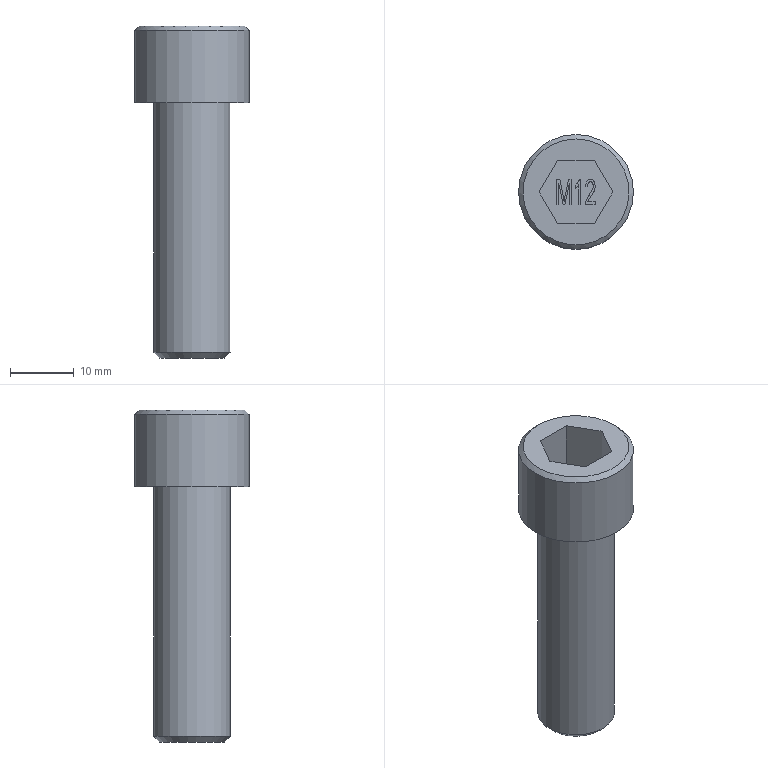Part | STEP file | EM11204000 | 1 solid | 43 faces | box 18 x 18 x 52 mm | volume 6858 mm3 | plane 33 | other 6 | cone 2 | cylinder 2 | commonest cylinder face diameters 12 x1 18 x1